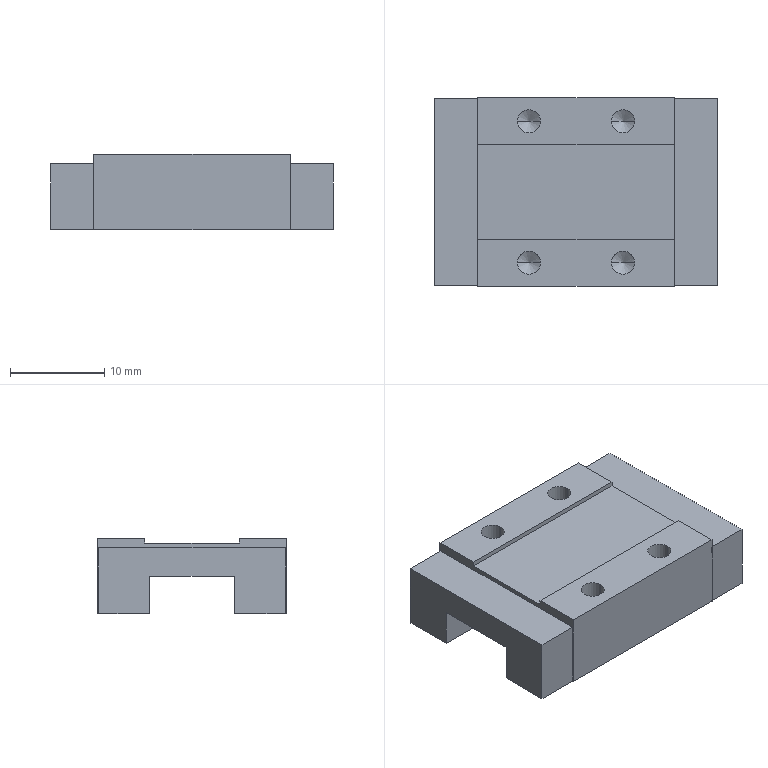Part | SolidWorks | features BaseBody 1 | 1 solid | 38 faces | box 30 x 20 x 8 mm | volume 3357 mm3 | plane 22 | cylinder 8 | cone 8 | commonest cylinder face diameters 2.459 x8
STEP:
#1=CARTESIAN_POINT('',(-38.836,-61.65,5.));
#2=VERTEX_POINT('',#1);
#3=CARTESIAN_POINT('',(-36.377,-61.65,5.));
#4=VERTEX_POINT('',#3);
#5=CARTESIAN_POINT('',(-37.606,-61.65,5.));
#6=DIRECTION('',(0.,0.,1.));
#7=DIRECTION('',(1.,0.,0.));
#8=AXIS2_PLACEMENT_3D('',#5,#6,#7);
#9=CIRCLE('',#8,1.23);
#10=EDGE_CURVE('',#2,#4,#9,.T.);
#11=ORIENTED_EDGE('',*,*,#10,.F.);
#12=CARTESIAN_POINT('',(-38.836,-61.65,8.));
#13=VERTEX_POINT('',#12);
#14=CARTESIAN_POINT('',(-38.836,-61.65,6.5));
#15=DIRECTION('',(0.,0.,1.));
#16=VECTOR('',#15,1000.);
#17=LINE('',#14,#16);
#18=EDGE_CURVE('',#2,#13,#17,.T.);
#19=ORIENTED_EDGE('',*,*,#18,.T.);
#20=CARTESIAN_POINT('',(-36.377,-61.65,8.));
#21=VERTEX_POINT('',#20);
#22=CARTESIAN_POINT('',(-37.606,-61.65,8.));
#23=DIRECTION('',(0.,0.,-1.));
#24=DIRECTION('',(1.,0.,0.));
#25=AXIS2_PLACEMENT_3D('',#22,#23,#24);
#26=CIRCLE('',#25,1.23);
#27=EDGE_CURVE('',#21,#13,#26,.T.);
#28=ORIENTED_EDGE('',*,*,#27,.F.);
#29=CARTESIAN_POINT('',(-36.377,-61.65,6.5));
#30=DIRECTION('',(0.,0.,1.));
#31=VECTOR('',#30,1000.);
#32=LINE('',#29,#31);
#33=EDGE_CURVE('',#4,#21,#32,.T.);
#34=ORIENTED_EDGE('',*,*,#33,.F.);
#35=EDGE_LOOP('',(#11,#19,#28,#34));
#36=FACE_OUTER_BOUND('',#35,.T.);
#37=CARTESIAN_POINT('',(-37.606,-61.65,6.5));
#38=DIRECTION('',(0.,0.,1.));
#39=DIRECTION('',(1.,0.,0.));
#40=AXIS2_PLACEMENT_3D('',#37,#38,#39);
#41=CYLINDRICAL_SURFACE('',#40,1.23);
#42=ADVANCED_FACE('',(#36),#41,.F.);
#43=CARTESIAN_POINT('',(-28.836,-61.65,5.));
#44=VERTEX_POINT('',#43);
#45=CARTESIAN_POINT('',(-26.377,-61.65,5.));
#46=VERTEX_POINT('',#45);
#47=CARTESIAN_POINT('',(-27.606,-61.65,5.));
#48=DIRECTION('',(0.,0.,1.));
#49=DIRECTION('',(1.,0.,0.));
#50=AXIS2_PLACEMENT_3D('',#47,#48,#49);
#51=CIRCLE('',#50,1.23);
#52=EDGE_CURVE('',#44,#46,#51,.T.);
#53=ORIENTED_EDGE('',*,*,#52,.F.);
#54=CARTESIAN_POINT('',(-28.836,-61.65,8.));
#55=VERTEX_POINT('',#54);
#56=CARTESIAN_POINT('',(-28.836,-61.65,6.5));
#57=DIRECTION('',(0.,0.,1.));
#58=VECTOR('',#57,1000.);
#59=LINE('',#56,#58);
#60=EDGE_CURVE('',#44,#55,#59,.T.);
#61=ORIENTED_EDGE('',*,*,#60,.T.);
#62=CARTESIAN_POINT('',(-26.377,-61.65,8.));
#63=VERTEX_POINT('',#62);
#64=CARTESIAN_POINT('',(-27.606,-61.65,8.));
#65=DIRECTION('',(0.,0.,-1.));
#66=DIRECTION('',(1.,0.,0.));
#67=AXIS2_PLACEMENT_3D('',#64,#65,#66);
#68=CIRCLE('',#67,1.23);
#69=EDGE_CURVE('',#63,#55,#68,.T.);
#70=ORIENTED_EDGE('',*,*,#69,.F.);
#71=CARTESIAN_POINT('',(-26.377,-61.65,6.5));
#72=DIRECTION('',(0.,0.,1.));
#73=VECTOR('',#72,1000.);
#74=LINE('',#71,#73);
#75=EDGE_CURVE('',#46,#63,#74,.T.);
#76=ORIENTED_EDGE('',*,*,#75,.F.);
#77=EDGE_LOOP('',(#53,#61,#70,#76));
#78=FACE_OUTER_BOUND('',#77,.T.);
#79=CARTESIAN_POINT('',(-27.606,-61.65,6.5));
#80=DIRECTION('',(0.,0.,1.));
#81=DIRECTION('',(1.,0.,0.));
#82=AXIS2_PLACEMENT_3D('',#79,#80,#81);
#83=CYLINDRICAL_SURFACE('',#82,1.23);
#84=ADVANCED_FACE('',(#78),#83,.F.);
#85=CARTESIAN_POINT('',(-38.836,-46.65,5.));
#86=VERTEX_POINT('',#85);
#87=CARTESIAN_POINT('',(-36.377,-46.65,5.));
#88=VERTEX_POINT('',#87);
#89=CARTESIAN_POINT('',(-37.606,-46.65,5.));
#90=DIRECTION('',(0.,0.,1.));
#91=DIRECTION('',(1.,0.,0.));
#92=AXIS2_PLACEMENT_3D('',#89,#90,#91);
#93=CIRCLE('',#92,1.23);
#94=EDGE_CURVE('',#86,#88,#93,.T.);
#95=ORIENTED_EDGE('',*,*,#94,.F.);
#96=CARTESIAN_POINT('',(-38.836,-46.65,8.));
#97=VERTEX_POINT('',#96);
#98=CARTESIAN_POINT('',(-38.836,-46.65,6.5));
#99=DIRECTION('',(0.,0.,1.));
#100=VECTOR('',#99,1000.);
#101=LINE('',#98,#100);
#102=EDGE_CURVE('',#86,#97,#101,.T.);
#103=ORIENTED_EDGE('',*,*,#102,.T.);
#104=CARTESIAN_POINT('',(-36.377,-46.65,8.));
#105=VERTEX_POINT('',#104);
#106=CARTESIAN_POINT('',(-37.606,-46.65,8.));
#107=DIRECTION('',(0.,0.,-1.));
#108=DIRECTION('',(1.,0.,0.));
#109=AXIS2_PLACEMENT_3D('',#106,#107,#108);
#110=CIRCLE('',#109,1.23);
#111=EDGE_CURVE('',#105,#97,#110,.T.);
#112=ORIENTED_EDGE('',*,*,#111,.F.);
#113=CARTESIAN_POINT('',(-36.377,-46.65,6.5));
#114=DIRECTION('',(0.,0.,1.));
#115=VECTOR('',#114,1000.);
#116=LINE('',#113,#115);
#117=EDGE_CURVE('',#88,#105,#116,.T.);
#118=ORIENTED_EDGE('',*,*,#117,.F.);
#119=EDGE_LOOP('',(#95,#103,#112,#118));
#120=FACE_OUTER_BOUND('',#119,.T.);
#121=CARTESIAN_POINT('',(-37.606,-46.65,6.5));
#122=DIRECTION('',(0.,0.,1.));
#123=DIRECTION('',(1.,0.,0.));
#124=AXIS2_PLACEMENT_3D('',#121,#122,#123);
#125=CYLINDRICAL_SURFACE('',#124,1.23);
#126=ADVANCED_FACE('',(#120),#125,.F.);
#127=CARTESIAN_POINT('',(-28.836,-46.65,5.));
#128=VERTEX_POINT('',#127);
#129=CARTESIAN_POINT('',(-26.377,-46.65,5.));
#130=VERTEX_POINT('',#129);
#131=CARTESIAN_POINT('',(-27.606,-46.65,5.));
#132=DIRECTION('',(0.,0.,1.));
#133=DIRECTION('',(1.,0.,0.));
#134=AXIS2_PLACEMENT_3D('',#131,#132,#133);
#135=CIRCLE('',#134,1.23);
#136=EDGE_CURVE('',#128,#130,#135,.T.);
#137=ORIENTED_EDGE('',*,*,#136,.F.);
#138=CARTESIAN_POINT('',(-28.836,-46.65,8.));
#139=VERTEX_POINT('',#138);
#140=CARTESIAN_POINT('',(-28.836,-46.65,6.5));
#141=DIRECTION('',(0.,0.,1.));
#142=VECTOR('',#141,1000.);
#143=LINE('',#140,#142);
#144=EDGE_CURVE('',#128,#139,#143,.T.);
#145=ORIENTED_EDGE('',*,*,#144,.T.);
#146=CARTESIAN_POINT('',(-26.377,-46.65,8.));
#147=VERTEX_POINT('',#146);
#148=CARTESIAN_POINT('',(-27.606,-46.65,8.));
#149=DIRECTION('',(0.,0.,-1.));
#150=DIRECTION('',(1.,0.,0.));
#151=AXIS2_PLACEMENT_3D('',#148,#149,#150);
#152=CIRCLE('',#151,1.23);
#153=EDGE_CURVE('',#147,#139,#152,.T.);
#154=ORIENTED_EDGE('',*,*,#153,.F.);
#155=CARTESIAN_POINT('',(-26.377,-46.65,6.5));
#156=DIRECTION('',(0.,0.,1.));
#157=VECTOR('',#156,1000.);
#158=LINE('',#155,#157);
#159=EDGE_CURVE('',#130,#147,#158,.T.);
#160=ORIENTED_EDGE('',*,*,#159,.F.);
#161=EDGE_LOOP('',(#137,#145,#154,#160));
#162=FACE_OUTER_BOUND('',#161,.T.);
#163=CARTESIAN_POINT('',(-27.606,-46.65,6.5));
#164=DIRECTION('',(0.,0.,1.));
#165=DIRECTION('',(1.,0.,0.));
#166=AXIS2_PLACEMENT_3D('',#163,#164,#165);
#167=CYLINDRICAL_SURFACE('',#166,1.23);
#168=ADVANCED_FACE('',(#162),#167,.F.);
#169=CARTESIAN_POINT('',(-37.606,-61.65,4.261));
#170=VERTEX_POINT('',#169);
#171=CARTESIAN_POINT('',(-36.377,-61.65,5.));
#172=DIRECTION('',(0.8572,0.,0.515));
#173=VECTOR('',#172,1000.);
#174=LINE('',#171,#173);
#175=EDGE_CURVE('',#170,#4,#174,.T.);
#176=ORIENTED_EDGE('',*,*,#175,.F.);
#177=CARTESIAN_POINT('',(-38.836,-61.65,5.));
#178=DIRECTION('',(-0.8572,0.,0.515));
#179=VECTOR('',#178,1000.);
#180=LINE('',#177,#179);
#181=EDGE_CURVE('',#170,#2,#180,.T.);
#182=ORIENTED_EDGE('',*,*,#181,.T.);
#183=ORIENTED_EDGE('',*,*,#10,.T.);
#184=EDGE_LOOP('',(#176,#182,#183));
#185=FACE_OUTER_BOUND('',#184,.T.);
#186=CARTESIAN_POINT('',(-37.606,-61.65,5.));
#187=DIRECTION('',(0.,0.,1.));
#188=DIRECTION('',(1.,0.,0.));
#189=AXIS2_PLACEMENT_3D('',#186,#187,#188);
#190=CONICAL_SURFACE('',#189,1.229,1.03);
#191=ADVANCED_FACE('',(#185),#190,.F.);
#192=CARTESIAN_POINT('',(-27.606,-61.65,4.261));
#193=VERTEX_POINT('',#192);
#194=CARTESIAN_POINT('',(-26.377,-61.65,5.));
#195=DIRECTION('',(0.8572,0.,0.515));
#196=VECTOR('',#195,1000.);
#197=LINE('',#194,#196);
#198=EDGE_CURVE('',#193,#46,#197,.T.);
#199=ORIENTED_EDGE('',*,*,#198,.F.);
#200=CARTESIAN_POINT('',(-28.836,-61.65,5.));
#201=DIRECTION('',(-0.8572,0.,0.515));
#202=VECTOR('',#201,1000.);
#203=LINE('',#200,#202);
#204=EDGE_CURVE('',#193,#44,#203,.T.);
#205=ORIENTED_EDGE('',*,*,#204,.T.);
#206=ORIENTED_EDGE('',*,*,#52,.T.);
#207=EDGE_LOOP('',(#199,#205,#206));
#208=FACE_OUTER_BOUND('',#207,.T.);
#209=CARTESIAN_POINT('',(-27.606,-61.65,5.));
#210=DIRECTION('',(0.,0.,1.));
#211=DIRECTION('',(1.,0.,0.));
#212=AXIS2_PLACEMENT_3D('',#209,#210,#211);
#213=CONICAL_SURFACE('',#212,1.229,1.03);
#214=ADVANCED_FACE('',(#208),#213,.F.);
#215=CARTESIAN_POINT('',(-37.606,-46.65,4.261));
#216=VERTEX_POINT('',#215);
#217=CARTESIAN_POINT('',(-36.377,-46.65,5.));
#218=DIRECTION('',(0.8572,0.,0.515));
#219=VECTOR('',#218,1000.);
#220=LINE('',#217,#219);
#221=EDGE_CURVE('',#216,#88,#220,.T.);
#222=ORIENTED_EDGE('',*,*,#221,.F.);
#223=CARTESIAN_POINT('',(-38.836,-46.65,5.));
#224=DIRECTION('',(-0.8572,0.,0.515));
#225=VECTOR('',#224,1000.);
#226=LINE('',#223,#225);
#227=EDGE_CURVE('',#216,#86,#226,.T.);
#228=ORIENTED_EDGE('',*,*,#227,.T.);
#229=ORIENTED_EDGE('',*,*,#94,.T.);
#230=EDGE_LOOP('',(#222,#228,#229));
#231=FACE_OUTER_BOUND('',#230,.T.);
#232=CARTESIAN_POINT('',(-37.606,-46.65,5.));
#233=DIRECTION('',(0.,0.,1.));
#234=DIRECTION('',(1.,0.,0.));
#235=AXIS2_PLACEMENT_3D('',#232,#233,#234);
#236=CONICAL_SURFACE('',#235,1.229,1.03);
#237=ADVANCED_FACE('',(#231),#236,.F.);
#238=CARTESIAN_POINT('',(-27.606,-46.65,4.261));
#239=VERTEX_POINT('',#238);
#240=CARTESIAN_POINT('',(-26.377,-46.65,5.));
#241=DIRECTION('',(0.8572,0.,0.515));
#242=VECTOR('',#241,1000.);
#243=LINE('',#240,#242);
#244=EDGE_CURVE('',#239,#130,#243,.T.);
#245=ORIENTED_EDGE('',*,*,#244,.F.);
#246=CARTESIAN_POINT('',(-28.836,-46.65,5.));
#247=DIRECTION('',(-0.8572,0.,0.515));
#248=VECTOR('',#247,1000.);
#249=LINE('',#246,#248);
#250=EDGE_CURVE('',#239,#128,#249,.T.);
#251=ORIENTED_EDGE('',*,*,#250,.T.);
#252=ORIENTED_EDGE('',*,*,#136,.T.);
#253=EDGE_LOOP('',(#245,#251,#252));
#254=FACE_OUTER_BOUND('',#253,.T.);
#255=CARTESIAN_POINT('',(-27.606,-46.65,5.));
#256=DIRECTION('',(0.,0.,1.));
#257=DIRECTION('',(1.,0.,0.));
#258=AXIS2_PLACEMENT_3D('',#255,#256,#257);
#259=CONICAL_SURFACE('',#258,1.229,1.03);
#260=ADVANCED_FACE('',(#254),#259,.F.);
#261=CARTESIAN_POINT('',(-47.606,-49.65,4.));
#262=VERTEX_POINT('',#261);
#263=CARTESIAN_POINT('',(-47.606,-58.65,4.));
#264=VERTEX_POINT('',#263);
#265=CARTESIAN_POINT('',(-47.606,-54.15,4.));
#266=DIRECTION('',(0.,-1.,0.));
#267=VECTOR('',#266,1000.);
#268=LINE('',#265,#267);
#269=EDGE_CURVE('',#262,#264,#268,.T.);
#270=ORIENTED_EDGE('',*,*,#269,.F.);
#271=CARTESIAN_POINT('',(-17.606,-49.65,4.));
#272=VERTEX_POINT('',#271);
#273=CARTESIAN_POINT('',(-32.606,-49.65,4.));
#274=DIRECTION('',(-1.,0.,0.));
#275=VECTOR('',#274,1000.);
#276=LINE('',#273,#275);
#277=EDGE_CURVE('',#272,#262,#276,.T.);
#278=ORIENTED_EDGE('',*,*,#277,.F.);
#279=CARTESIAN_POINT('',(-17.606,-58.65,4.));
#280=VERTEX_POINT('',#279);
#281=CARTESIAN_POINT('',(-17.606,-54.15,4.));
#282=DIRECTION('',(0.,1.,0.));
#283=VECTOR('',#282,1000.);
#284=LINE('',#281,#283);
#285=EDGE_CURVE('',#280,#272,#284,.T.);
#286=ORIENTED_EDGE('',*,*,#285,.F.);
#287=CARTESIAN_POINT('',(-32.606,-58.65,4.));
#288=DIRECTION('',(1.,0.,0.));
#289=VECTOR('',#288,1000.);
#290=LINE('',#287,#289);
#291=EDGE_CURVE('',#264,#280,#290,.T.);
#292=ORIENTED_EDGE('',*,*,#291,.F.);
#293=EDGE_LOOP('',(#270,#278,#286,#292));
#294=FACE_OUTER_BOUND('',#293,.T.);
#295=CARTESIAN_POINT('',(-32.606,-54.15,4.));
#296=DIRECTION('',(0.,0.,1.));
#297=DIRECTION('',(1.,0.,0.));
#298=AXIS2_PLACEMENT_3D('',#295,#296,#297);
#299=PLANE('',#298);
#300=ADVANCED_FACE('',(#294),#299,.F.);
#301=CARTESIAN_POINT('',(-17.606,-58.65,0.));
#302=VERTEX_POINT('',#301);
#303=CARTESIAN_POINT('',(-17.606,-58.65,0.));
#304=DIRECTION('',(0.,0.,1.));
#305=VECTOR('',#304,1000.);
#306=LINE('',#303,#305);
#307=EDGE_CURVE('',#302,#280,#306,.T.);
#308=ORIENTED_EDGE('',*,*,#307,.F.);
#309=CARTESIAN_POINT('',(-47.606,-58.65,0.));
#310=VERTEX_POINT('',#309);
#311=CARTESIAN_POINT('',(-17.606,-58.65,0.));
#312=DIRECTION('',(1.,0.,0.));
#313=VECTOR('',#312,1000.);
#314=LINE('',#311,#313);
#315=EDGE_CURVE('',#310,#302,#314,.T.);
#316=ORIENTED_EDGE('',*,*,#315,.F.);
#317=CARTESIAN_POINT('',(-47.606,-58.65,0.));
#318=DIRECTION('',(0.,0.,-1.));
#319=VECTOR('',#318,1000.);
#320=LINE('',#317,#319);
#321=EDGE_CURVE('',#264,#310,#320,.T.);
#322=ORIENTED_EDGE('',*,*,#321,.F.);
#323=ORIENTED_EDGE('',*,*,#291,.T.);
#324=EDGE_LOOP('',(#308,#316,#322,#323));
#325=FACE_OUTER_BOUND('',#324,.T.);
#326=CARTESIAN_POINT('',(-17.606,-58.65,0.));
#327=DIRECTION('',(0.,-1.,0.));
#328=DIRECTION('',(0.,0.,-1.));
#329=AXIS2_PLACEMENT_3D('',#326,#327,#328);
#330=PLANE('',#329);
#331=ADVANCED_FACE('',(#325),#330,.F.);
#332=CARTESIAN_POINT('',(-47.606,-64.05,0.));
#333=VERTEX_POINT('',#332);
#334=CARTESIAN_POINT('',(-47.606,-64.05,7.));
#335=VERTEX_POINT('',#334);
#336=CARTESIAN_POINT('',(-47.606,-64.05,0.));
#337=DIRECTION('',(0.,0.,1.));
#338=VECTOR('',#337,1000.);
#339=LINE('',#336,#338);
#340=EDGE_CURVE('',#333,#335,#339,.T.);
#341=ORIENTED_EDGE('',*,*,#340,.T.);
#342=CARTESIAN_POINT('',(-47.606,-44.25,7.));
#343=VERTEX_POINT('',#342);
#344=CARTESIAN_POINT('',(-47.606,-64.15,7.));
#345=DIRECTION('',(0.,1.,0.));
#346=VECTOR('',#345,1000.);
#347=LINE('',#344,#346);
#348=EDGE_CURVE('',#335,#343,#347,.T.);
#349=ORIENTED_EDGE('',*,*,#348,.T.);
#350=CARTESIAN_POINT('',(-47.606,-44.25,0.));
#351=VERTEX_POINT('',#350);
#352=CARTESIAN_POINT('',(-47.606,-44.25,0.));
#353=DIRECTION('',(0.,0.,-1.));
#354=VECTOR('',#353,1000.);
#355=LINE('',#352,#354);
#356=EDGE_CURVE('',#343,#351,#355,.T.);
#357=ORIENTED_EDGE('',*,*,#356,.T.);
#358=CARTESIAN_POINT('',(-47.606,-49.65,0.));
#359=VERTEX_POINT('',#358);
#360=CARTESIAN_POINT('',(-47.606,-64.15,0.));
#361=DIRECTION('',(0.,-1.,0.));
#362=VECTOR('',#361,1000.);
#363=LINE('',#360,#362);
#364=EDGE_CURVE('',#351,#359,#363,.T.);
#365=ORIENTED_EDGE('',*,*,#364,.T.);
#366=CARTESIAN_POINT('',(-47.606,-49.65,0.));
#367=DIRECTION('',(0.,0.,1.));
#368=VECTOR('',#367,1000.);
#369=LINE('',#366,#368);
#370=EDGE_CURVE('',#359,#262,#369,.T.);
#371=ORIENTED_EDGE('',*,*,#370,.T.);
#372=ORIENTED_EDGE('',*,*,#269,.T.);
#373=ORIENTED_EDGE('',*,*,#321,.T.);
#374=CARTESIAN_POINT('',(-47.606,-64.15,0.));
#375=DIRECTION('',(0.,-1.,0.));
#376=VECTOR('',#375,1000.);
#377=LINE('',#374,#376);
#378=EDGE_CURVE('',#310,#333,#377,.T.);
#379=ORIENTED_EDGE('',*,*,#378,.T.);
#380=EDGE_LOOP('',(#341,#349,#357,#365,#371,#372,#373,#379));
#381=FACE_OUTER_BOUND('',#380,.T.);
#382=CARTESIAN_POINT('',(-47.606,-64.15,0.));
#383=DIRECTION('',(-1.,0.,0.));
#384=DIRECTION('',(0.,0.,1.));
#385=AXIS2_PLACEMENT_3D('',#382,#383,#384);
#386=PLANE('',#385);
#387=ADVANCED_FACE('',(#381),#386,.T.);
#388=ORIENTED_EDGE('',*,*,#370,.F.);
#389=CARTESIAN_POINT('',(-17.606,-49.65,0.));
#390=VERTEX_POINT('',#389);
#391=CARTESIAN_POINT('',(-47.606,-49.65,0.));
#392=DIRECTION('',(-1.,0.,0.));
#393=VECTOR('',#392,1000.);
#394=LINE('',#391,#393);
#395=EDGE_CURVE('',#390,#359,#394,.T.);
#396=ORIENTED_EDGE('',*,*,#395,.F.);
#397=CARTESIAN_POINT('',(-17.606,-49.65,0.));
#398=DIRECTION('',(0.,0.,-1.));
#399=VECTOR('',#398,1000.);
#400=LINE('',#397,#399);
#401=EDGE_CURVE('',#272,#390,#400,.T.);
#402=ORIENTED_EDGE('',*,*,#401,.F.);
#403=ORIENTED_EDGE('',*,*,#277,.T.);
#404=EDGE_LOOP('',(#388,#396,#402,#403));
#405=FACE_OUTER_BOUND('',#404,.T.);
#406=CARTESIAN_POINT('',(-47.606,-49.65,0.));
#407=DIRECTION('',(0.,1.,0.));
#408=DIRECTION('',(0.,0.,1.));
#409=AXIS2_PLACEMENT_3D('',#406,#407,#408);
#410=PLANE('',#409);
#411=ADVANCED_FACE('',(#405),#410,.F.);
#412=ORIENTED_EDGE('',*,*,#401,.T.);
#413=CARTESIAN_POINT('',(-17.606,-44.25,0.));
#414=VERTEX_POINT('',#413);
#415=CARTESIAN_POINT('',(-17.606,-44.15,0.));
#416=DIRECTION('',(0.,1.,0.));
#417=VECTOR('',#416,1000.);
#418=LINE('',#415,#417);
#419=EDGE_CURVE('',#390,#414,#418,.T.);
#420=ORIENTED_EDGE('',*,*,#419,.T.);
#421=CARTESIAN_POINT('',(-17.606,-44.25,7.));
#422=VERTEX_POINT('',#421);
#423=CARTESIAN_POINT('',(-17.606,-44.25,0.));
#424=DIRECTION('',(0.,0.,1.));
#425=VECTOR('',#424,1000.);
#426=LINE('',#423,#425);
#427=EDGE_CURVE('',#414,#422,#426,.T.);
#428=ORIENTED_EDGE('',*,*,#427,.T.);
#429=CARTESIAN_POINT('',(-17.606,-64.05,7.));
#430=VERTEX_POINT('',#429);
#431=CARTESIAN_POINT('',(-17.606,-44.15,7.));
#432=DIRECTION('',(0.,-1.,0.));
#433=VECTOR('',#432,1000.);
#434=LINE('',#431,#433);
#435=EDGE_CURVE('',#422,#430,#434,.T.);
#436=ORIENTED_EDGE('',*,*,#435,.T.);
#437=CARTESIAN_POINT('',(-17.606,-64.05,0.));
#438=VERTEX_POINT('',#437);
#439=CARTESIAN_POINT('',(-17.606,-64.05,0.));
#440=DIRECTION('',(0.,0.,-1.));
#441=VECTOR('',#440,1000.);
#442=LINE('',#439,#441);
#443=EDGE_CURVE('',#430,#438,#442,.T.);
#444=ORIENTED_EDGE('',*,*,#443,.T.);
#445=CARTESIAN_POINT('',(-17.606,-44.15,0.));
#446=DIRECTION('',(0.,1.,0.));
#447=VECTOR('',#446,1000.);
#448=LINE('',#445,#447);
#449=EDGE_CURVE('',#438,#302,#448,.T.);
#450=ORIENTED_EDGE('',*,*,#449,.T.);
#451=ORIENTED_EDGE('',*,*,#307,.T.);
#452=ORIENTED_EDGE('',*,*,#285,.T.);
#453=EDGE_LOOP('',(#412,#420,#428,#436,#444,#450,#451,#452));
#454=FACE_OUTER_BOUND('',#453,.T.);
#455=CARTESIAN_POINT('',(-17.606,-44.15,0.));
#456=DIRECTION('',(1.,0.,0.));
#457=DIRECTION('',(0.,0.,-1.));
#458=AXIS2_PLACEMENT_3D('',#455,#456,#457);
#459=PLANE('',#458);
#460=ADVANCED_FACE('',(#454),#459,.T.);
#461=ORIENTED_EDGE('',*,*,#378,.F.);
#462=ORIENTED_EDGE('',*,*,#315,.T.);
#463=ORIENTED_EDGE('',*,*,#449,.F.);
#464=CARTESIAN_POINT('',(-22.206,-64.05,0.));
#465=VERTEX_POINT('',#464);
#466=CARTESIAN_POINT('',(-32.606,-64.05,0.));
#467=DIRECTION('',(1.,0.,0.));
#468=VECTOR('',#467,1000.);
#469=LINE('',#466,#468);
#470=EDGE_CURVE('',#465,#438,#469,.T.);
#471=ORIENTED_EDGE('',*,*,#470,.F.);
#472=CARTESIAN_POINT('',(-22.206,-64.15,0.));
#473=VERTEX_POINT('',#472);
#474=CARTESIAN_POINT('',(-22.206,-44.15,0.));
#475=DIRECTION('',(0.,-1.,0.));
#476=VECTOR('',#475,1000.);
#477=LINE('',#474,#476);
#478=EDGE_CURVE('',#465,#473,#477,.T.);
#479=ORIENTED_EDGE('',*,*,#478,.T.);
#480=CARTESIAN_POINT('',(-43.006,-64.15,0.));
#481=VERTEX_POINT('',#480);
#482=CARTESIAN_POINT('',(-32.606,-64.15,0.));
#483=DIRECTION('',(1.,0.,0.));
#484=VECTOR('',#483,1000.);
#485=LINE('',#482,#484);
#486=EDGE_CURVE('',#481,#473,#485,.T.);
#487=ORIENTED_EDGE('',*,*,#486,.F.);
#488=CARTESIAN_POINT('',(-43.006,-64.05,0.));
#489=VERTEX_POINT('',#488);
#490=CARTESIAN_POINT('',(-43.006,-64.15,0.));
#491=DIRECTION('',(0.,1.,0.));
#492=VECTOR('',#491,1000.);
#493=LINE('',#490,#492);
#494=EDGE_CURVE('',#481,#489,#493,.T.);
#495=ORIENTED_EDGE('',*,*,#494,.T.);
#496=CARTESIAN_POINT('',(-32.606,-64.05,0.));
#497=DIRECTION('',(1.,0.,0.));
#498=VECTOR('',#497,1000.);
#499=LINE('',#496,#498);
#500=EDGE_CURVE('',#333,#489,#499,.T.);
#501=ORIENTED_EDGE('',*,*,#500,.F.);
#502=EDGE_LOOP('',(#461,#462,#463,#471,#479,#487,#495,#501));
#503=FACE_OUTER_BOUND('',#502,.T.);
#504=CARTESIAN_POINT('',(-32.606,-54.15,0.));
#505=DIRECTION('',(0.,0.,1.));
#506=DIRECTION('',(1.,0.,0.));
#507=AXIS2_PLACEMENT_3D('',#504,#505,#506);
#508=PLANE('',#507);
#509=ADVANCED_FACE('',(#503),#508,.F.);
#510=CARTESIAN_POINT('',(-43.006,-64.05,7.));
#511=VERTEX_POINT('',#510);
#512=CARTESIAN_POINT('',(-45.306,-64.05,7.));
#513=DIRECTION('',(1.,0.,0.));
#514=VECTOR('',#513,1000.);
#515=LINE('',#512,#514);
#516=EDGE_CURVE('',#335,#511,#515,.T.);
#517=ORIENTED_EDGE('',*,*,#516,.T.);
#518=CARTESIAN_POINT('',(-43.006,-44.25,7.));
#519=VERTEX_POINT('',#518);
#520=CARTESIAN_POINT('',(-43.006,-54.15,7.));
#521=DIRECTION('',(0.,1.,0.));
#522=VECTOR('',#521,1000.);
#523=LINE('',#520,#522);
#524=EDGE_CURVE('',#511,#519,#523,.T.);
#525=ORIENTED_EDGE('',*,*,#524,.T.);
#526=CARTESIAN_POINT('',(-45.306,-44.25,7.));
#527=DIRECTION('',(-1.,0.,0.));
#528=VECTOR('',#527,1000.);
#529=LINE('',#526,#528);
#530=EDGE_CURVE('',#519,#343,#529,.T.);
#531=ORIENTED_EDGE('',*,*,#530,.T.);
#532=ORIENTED_EDGE('',*,*,#348,.F.);
#533=EDGE_LOOP('',(#517,#525,#531,#532));
#534=FACE_OUTER_BOUND('',#533,.T.);
#535=CARTESIAN_POINT('',(-45.306,-54.15,7.));
#536=DIRECTION('',(0.,0.,1.));
#537=DIRECTION('',(1.,0.,0.));
#538=AXIS2_PLACEMENT_3D('',#535,#536,#537);
#539=PLANE('',#538);
#540=ADVANCED_FACE('',(#534),#539,.T.);
#541=ORIENTED_EDGE('',*,*,#500,.T.);
#542=CARTESIAN_POINT('',(-43.006,-64.05,3.5));
#543=DIRECTION('',(0.,0.,-1.));
#544=VECTOR('',#543,1000.);
#545=LINE('',#542,#544);
#546=EDGE_CURVE('',#511,#489,#545,.T.);
#547=ORIENTED_EDGE('',*,*,#546,.F.);
#548=ORIENTED_EDGE('',*,*,#516,.F.);
#549=ORIENTED_EDGE('',*,*,#340,.F.);
#550=EDGE_LOOP('',(#541,#547,#548,#549));
#551=FACE_OUTER_BOUND('',#550,.T.);
#552=CARTESIAN_POINT('',(-45.306,-64.05,3.5));
#553=DIRECTION('',(0.,1.,0.));
#554=DIRECTION('',(0.,0.,1.));
#555=AXIS2_PLACEMENT_3D('',#552,#553,#554);
#556=PLANE('',#555);
#557=ADVANCED_FACE('',(#551),#556,.F.);
#558=CARTESIAN_POINT('',(-43.006,-44.15,0.));
#559=VERTEX_POINT('',#558);
#560=CARTESIAN_POINT('',(-43.006,-44.25,0.));
#561=VERTEX_POINT('',#560);
#562=CARTESIAN_POINT('',(-43.006,-54.15,0.));
#563=DIRECTION('',(0.,-1.,0.));
#564=VECTOR('',#563,1000.);
#565=LINE('',#562,#564);
#566=EDGE_CURVE('',#559,#561,#565,.T.);
#567=ORIENTED_EDGE('',*,*,#566,.F.);
#568=CARTESIAN_POINT('',(-22.206,-44.15,0.));
#569=VERTEX_POINT('',#568);
#570=CARTESIAN_POINT('',(-32.606,-44.15,0.));
#571=DIRECTION('',(-1.,0.,0.));
#572=VECTOR('',#571,1000.);
#573=LINE('',#570,#572);
#574=EDGE_CURVE('',#569,#559,#573,.T.);
#575=ORIENTED_EDGE('',*,*,#574,.F.);
#576=CARTESIAN_POINT('',(-22.206,-44.25,0.));
#577=VERTEX_POINT('',#576);
#578=CARTESIAN_POINT('',(-22.206,-44.15,0.));
#579=DIRECTION('',(0.,-1.,0.));
#580=VECTOR('',#579,1000.);
#581=LINE('',#578,#580);
#582=EDGE_CURVE('',#569,#577,#581,.T.);
#583=ORIENTED_EDGE('',*,*,#582,.T.);
#584=CARTESIAN_POINT('',(-32.606,-44.25,0.));
#585=DIRECTION('',(-1.,0.,0.));
#586=VECTOR('',#585,1000.);
#587=LINE('',#584,#586);
#588=EDGE_CURVE('',#414,#577,#587,.T.);
#589=ORIENTED_EDGE('',*,*,#588,.F.);
#590=ORIENTED_EDGE('',*,*,#419,.F.);
#591=ORIENTED_EDGE('',*,*,#395,.T.);
#592=ORIENTED_EDGE('',*,*,#364,.F.);
#593=CARTESIAN_POINT('',(-32.606,-44.25,0.));
#594=DIRECTION('',(-1.,0.,0.));
#595=VECTOR('',#594,1000.);
#596=LINE('',#593,#595);
#597=EDGE_CURVE('',#561,#351,#596,.T.);
#598=ORIENTED_EDGE('',*,*,#597,.F.);
#599=EDGE_LOOP('',(#567,#575,#583,#589,#590,#591,#592,#598));
#600=FACE_OUTER_BOUND('',#599,.T.);
#601=CARTESIAN_POINT('',(-32.606,-54.15,0.));
#602=DIRECTION('',(0.,0.,1.));
#603=DIRECTION('',(1.,0.,0.));
#604=AXIS2_PLACEMENT_3D('',#601,#602,#603);
#605=PLANE('',#604);
#606=ADVANCED_FACE('',(#600),#605,.F.);
#607=ORIENTED_EDGE('',*,*,#530,.F.);
#608=CARTESIAN_POINT('',(-43.006,-44.25,3.5));
#609=DIRECTION('',(0.,0.,-1.));
#610=VECTOR('',#609,1000.);
#611=LINE('',#608,#610);
#612=EDGE_CURVE('',#519,#561,#611,.T.);
#613=ORIENTED_EDGE('',*,*,#612,.T.);
#614=ORIENTED_EDGE('',*,*,#597,.T.);
#615=ORIENTED_EDGE('',*,*,#356,.F.);
#616=EDGE_LOOP('',(#607,#613,#614,#615));
#617=FACE_OUTER_BOUND('',#616,.T.);
#618=CARTESIAN_POINT('',(-45.306,-44.25,3.5));
#619=DIRECTION('',(0.,1.,0.));
#620=DIRECTION('',(0.,0.,1.));
#621=AXIS2_PLACEMENT_3D('',#618,#619,#620);
#622=PLANE('',#621);
#623=ADVANCED_FACE('',(#617),#622,.T.);
#624=CARTESIAN_POINT('',(-22.206,-64.05,7.));
#625=VERTEX_POINT('',#624);
#626=CARTESIAN_POINT('',(-22.206,-64.05,3.5));
#627=DIRECTION('',(0.,0.,1.));
#628=VECTOR('',#627,1000.);
#629=LINE('',#626,#628);
#630=EDGE_CURVE('',#465,#625,#629,.T.);
#631=ORIENTED_EDGE('',*,*,#630,.F.);
#632=ORIENTED_EDGE('',*,*,#470,.T.);
#633=ORIENTED_EDGE('',*,*,#443,.F.);
#634=CARTESIAN_POINT('',(-19.906,-64.05,7.));
#635=DIRECTION('',(1.,0.,0.));
#636=VECTOR('',#635,1000.);
#637=LINE('',#634,#636);
#638=EDGE_CURVE('',#625,#430,#637,.T.);
#639=ORIENTED_EDGE('',*,*,#638,.F.);
#640=EDGE_LOOP('',(#631,#632,#633,#639));
#641=FACE_OUTER_BOUND('',#640,.T.);
#642=CARTESIAN_POINT('',(-19.906,-64.05,3.5));
#643=DIRECTION('',(0.,1.,0.));
#644=DIRECTION('',(0.,0.,1.));
#645=AXIS2_PLACEMENT_3D('',#642,#643,#644);
#646=PLANE('',#645);
#647=ADVANCED_FACE('',(#641),#646,.F.);
#648=ORIENTED_EDGE('',*,*,#638,.T.);
#649=ORIENTED_EDGE('',*,*,#435,.F.);
#650=CARTESIAN_POINT('',(-22.206,-44.25,7.));
#651=VERTEX_POINT('',#650);
#652=CARTESIAN_POINT('',(-19.906,-44.25,7.));
#653=DIRECTION('',(-1.,0.,0.));
#654=VECTOR('',#653,1000.);
#655=LINE('',#652,#654);
#656=EDGE_CURVE('',#422,#651,#655,.T.);
#657=ORIENTED_EDGE('',*,*,#656,.T.);
#658=CARTESIAN_POINT('',(-22.206,-54.15,7.));
#659=DIRECTION('',(0.,-1.,0.));
#660=VECTOR('',#659,1000.);
#661=LINE('',#658,#660);
#662=EDGE_CURVE('',#651,#625,#661,.T.);
#663=ORIENTED_EDGE('',*,*,#662,.T.);
#664=EDGE_LOOP('',(#648,#649,#657,#663));
#665=FACE_OUTER_BOUND('',#664,.T.);
#666=CARTESIAN_POINT('',(-19.906,-54.15,7.));
#667=DIRECTION('',(0.,0.,1.));
#668=DIRECTION('',(1.,0.,0.));
#669=AXIS2_PLACEMENT_3D('',#666,#667,#668);
#670=PLANE('',#669);
#671=ADVANCED_FACE('',(#665),#670,.T.);
#672=CARTESIAN_POINT('',(-22.206,-44.25,3.5));
#673=DIRECTION('',(0.,0.,1.));
#674=VECTOR('',#673,1000.);
#675=LINE('',#672,#674);
#676=EDGE_CURVE('',#577,#651,#675,.T.);
#677=ORIENTED_EDGE('',*,*,#676,.T.);
#678=ORIENTED_EDGE('',*,*,#656,.F.);
#679=ORIENTED_EDGE('',*,*,#427,.F.);
#680=ORIENTED_EDGE('',*,*,#588,.T.);
#681=EDGE_LOOP('',(#677,#678,#679,#680));
#682=FACE_OUTER_BOUND('',#681,.T.);
#683=CARTESIAN_POINT('',(-19.906,-44.25,3.5));
#684=DIRECTION('',(0.,1.,0.));
#685=DIRECTION('',(0.,0.,1.));
#686=AXIS2_PLACEMENT_3D('',#683,#684,#685);
#687=PLANE('',#686);
#688=ADVANCED_FACE('',(#682),#687,.T.);
#689=CARTESIAN_POINT('',(-22.206,-64.15,8.));
#690=VERTEX_POINT('',#689);
#691=CARTESIAN_POINT('',(-22.206,-64.15,0.));
#692=DIRECTION('',(0.,0.,1.));
#693=VECTOR('',#692,1000.);
#694=LINE('',#691,#693);
#695=EDGE_CURVE('',#473,#690,#694,.T.);
#696=ORIENTED_EDGE('',*,*,#695,.T.);
#697=CARTESIAN_POINT('',(-43.006,-64.15,8.));
#698=VERTEX_POINT('',#697);
#699=CARTESIAN_POINT('',(-17.606,-64.15,8.));
#700=DIRECTION('',(-1.,0.,0.));
#701=VECTOR('',#700,1000.);
#702=LINE('',#699,#701);
#703=EDGE_CURVE('',#690,#698,#702,.T.);
#704=ORIENTED_EDGE('',*,*,#703,.T.);
#705=CARTESIAN_POINT('',(-43.006,-64.15,0.));
#706=DIRECTION('',(0.,0.,-1.));
#707=VECTOR('',#706,1000.);
#708=LINE('',#705,#707);
#709=EDGE_CURVE('',#698,#481,#708,.T.);
#710=ORIENTED_EDGE('',*,*,#709,.T.);
#711=ORIENTED_EDGE('',*,*,#486,.T.);
#712=EDGE_LOOP('',(#696,#704,#710,#711));
#713=FACE_OUTER_BOUND('',#712,.T.);
#714=CARTESIAN_POINT('',(-17.606,-64.15,0.));
#715=DIRECTION('',(0.,-1.,0.));
#716=DIRECTION('',(0.,0.,-1.));
#717=AXIS2_PLACEMENT_3D('',#714,#715,#716);
#718=PLANE('',#717);
#719=ADVANCED_FACE('',(#713),#718,.T.);
#720=CARTESIAN_POINT('',(-43.006,-49.15,7.5));
#721=VERTEX_POINT('',#720);
#722=CARTESIAN_POINT('',(-43.006,-59.15,7.5));
#723=VERTEX_POINT('',#722);
#724=CARTESIAN_POINT('',(-43.006,-64.15,7.5));
#725=DIRECTION('',(0.,-1.,0.));
#726=VECTOR('',#725,1000.);
#727=LINE('',#724,#726);
#728=EDGE_CURVE('',#721,#723,#727,.T.);
#729=ORIENTED_EDGE('',*,*,#728,.F.);
#730=CARTESIAN_POINT('',(-43.006,-49.15,8.));
#731=VERTEX_POINT('',#730);
#732=CARTESIAN_POINT('',(-43.006,-49.15,8.));
#733=DIRECTION('',(0.,0.,1.));
#734=VECTOR('',#733,1000.);
#735=LINE('',#732,#734);
#736=EDGE_CURVE('',#721,#731,#735,.T.);
#737=ORIENTED_EDGE('',*,*,#736,.T.);
#738=CARTESIAN_POINT('',(-43.006,-44.15,8.));
#739=VERTEX_POINT('',#738);
#740=CARTESIAN_POINT('',(-43.006,-64.15,8.));
#741=DIRECTION('',(0.,-1.,0.));
#742=VECTOR('',#741,1000.);
#743=LINE('',#740,#742);
#744=EDGE_CURVE('',#739,#731,#743,.T.);
#745=ORIENTED_EDGE('',*,*,#744,.F.);
#746=CARTESIAN_POINT('',(-43.006,-44.15,8.));
#747=DIRECTION('',(0.,0.,1.));
#748=VECTOR('',#747,1000.);
#749=LINE('',#746,#748);
#750=EDGE_CURVE('',#559,#739,#749,.T.);
#751=ORIENTED_EDGE('',*,*,#750,.F.);
#752=ORIENTED_EDGE('',*,*,#566,.T.);
#753=ORIENTED_EDGE('',*,*,#612,.F.);
#754=ORIENTED_EDGE('',*,*,#524,.F.);
#755=ORIENTED_EDGE('',*,*,#546,.T.);
#756=ORIENTED_EDGE('',*,*,#494,.F.);
#757=ORIENTED_EDGE('',*,*,#709,.F.);
#758=CARTESIAN_POINT('',(-43.006,-59.15,8.));
#759=VERTEX_POINT('',#758);
#760=CARTESIAN_POINT('',(-43.006,-64.15,8.));
#761=DIRECTION('',(0.,-1.,0.));
#762=VECTOR('',#761,1000.);
#763=LINE('',#760,#762);
#764=EDGE_CURVE('',#759,#698,#763,.T.);
#765=ORIENTED_EDGE('',*,*,#764,.F.);
#766=CARTESIAN_POINT('',(-43.006,-59.15,8.));
#767=DIRECTION('',(0.,0.,-1.));
#768=VECTOR('',#767,1000.);
#769=LINE('',#766,#768);
#770=EDGE_CURVE('',#759,#723,#769,.T.);
#771=ORIENTED_EDGE('',*,*,#770,.T.);
#772=EDGE_LOOP('',(#729,#737,#745,#751,#752,#753,#754,#755,#756,#757,#765,#771));
#773=FACE_OUTER_BOUND('',#772,.T.);
#774=CARTESIAN_POINT('',(-43.006,-64.15,8.));
#775=DIRECTION('',(1.,0.,0.));
#776=DIRECTION('',(0.,0.,-1.));
#777=AXIS2_PLACEMENT_3D('',#774,#775,#776);
#778=PLANE('',#777);
#779=ADVANCED_FACE('',(#773),#778,.F.);
#780=CARTESIAN_POINT('',(-22.206,-44.15,8.));
#781=VERTEX_POINT('',#780);
#782=CARTESIAN_POINT('',(-22.206,-44.15,0.));
#783=DIRECTION('',(0.,0.,-1.));
#784=VECTOR('',#783,1000.);
#785=LINE('',#782,#784);
#786=EDGE_CURVE('',#781,#569,#785,.T.);
#787=ORIENTED_EDGE('',*,*,#786,.T.);
#788=ORIENTED_EDGE('',*,*,#574,.T.);
#789=ORIENTED_EDGE('',*,*,#750,.T.);
#790=CARTESIAN_POINT('',(-47.606,-44.15,8.));
#791=DIRECTION('',(1.,0.,0.));
#792=VECTOR('',#791,1000.);
#793=LINE('',#790,#792);
#794=EDGE_CURVE('',#739,#781,#793,.T.);
#795=ORIENTED_EDGE('',*,*,#794,.T.);
#796=EDGE_LOOP('',(#787,#788,#789,#795));
#797=FACE_OUTER_BOUND('',#796,.T.);
#798=CARTESIAN_POINT('',(-47.606,-44.15,0.));
#799=DIRECTION('',(0.,1.,0.));
#800=DIRECTION('',(0.,0.,1.));
#801=AXIS2_PLACEMENT_3D('',#798,#799,#800);
#802=PLANE('',#801);
#803=ADVANCED_FACE('',(#797),#802,.T.);
#804=CARTESIAN_POINT('',(-22.206,-59.15,8.));
#805=VERTEX_POINT('',#804);
#806=CARTESIAN_POINT('',(-22.206,-44.15,8.));
#807=DIRECTION('',(0.,1.,0.));
#808=VECTOR('',#807,1000.);
#809=LINE('',#806,#808);
#810=EDGE_CURVE('',#690,#805,#809,.T.);
#811=ORIENTED_EDGE('',*,*,#810,.F.);
#812=ORIENTED_EDGE('',*,*,#695,.F.);
#813=ORIENTED_EDGE('',*,*,#478,.F.);
#814=ORIENTED_EDGE('',*,*,#630,.T.);
#815=ORIENTED_EDGE('',*,*,#662,.F.);
#816=ORIENTED_EDGE('',*,*,#676,.F.);
#817=ORIENTED_EDGE('',*,*,#582,.F.);
#818=ORIENTED_EDGE('',*,*,#786,.F.);
#819=CARTESIAN_POINT('',(-22.206,-49.15,8.));
#820=VERTEX_POINT('',#819);
#821=CARTESIAN_POINT('',(-22.206,-44.15,8.));
#822=DIRECTION('',(0.,1.,0.));
#823=VECTOR('',#822,1000.);
#824=LINE('',#821,#823);
#825=EDGE_CURVE('',#820,#781,#824,.T.);
#826=ORIENTED_EDGE('',*,*,#825,.F.);
#827=CARTESIAN_POINT('',(-22.206,-49.15,7.5));
#828=VERTEX_POINT('',#827);
#829=CARTESIAN_POINT('',(-22.206,-49.15,8.));
#830=DIRECTION('',(0.,0.,-1.));
#831=VECTOR('',#830,1000.);
#832=LINE('',#829,#831);
#833=EDGE_CURVE('',#820,#828,#832,.T.);
#834=ORIENTED_EDGE('',*,*,#833,.T.);
#835=CARTESIAN_POINT('',(-22.206,-59.15,7.5));
#836=VERTEX_POINT('',#835);
#837=CARTESIAN_POINT('',(-22.206,-44.15,7.5));
#838=DIRECTION('',(0.,1.,0.));
#839=VECTOR('',#838,1000.);
#840=LINE('',#837,#839);
#841=EDGE_CURVE('',#836,#828,#840,.T.);
#842=ORIENTED_EDGE('',*,*,#841,.F.);
#843=CARTESIAN_POINT('',(-22.206,-59.15,8.));
#844=DIRECTION('',(0.,0.,1.));
#845=VECTOR('',#844,1000.);
#846=LINE('',#843,#845);
#847=EDGE_CURVE('',#836,#805,#846,.T.);
#848=ORIENTED_EDGE('',*,*,#847,.T.);
#849=EDGE_LOOP('',(#811,#812,#813,#814,#815,#816,#817,#818,#826,#834,#842,#848));
#850=FACE_OUTER_BOUND('',#849,.T.);
#851=CARTESIAN_POINT('',(-22.206,-44.15,8.));
#852=DIRECTION('',(-1.,0.,0.));
#853=DIRECTION('',(0.,0.,1.));
#854=AXIS2_PLACEMENT_3D('',#851,#852,#853);
#855=PLANE('',#854);
#856=ADVANCED_FACE('',(#850),#855,.F.);
#857=ORIENTED_EDGE('',*,*,#27,.T.);
#858=CARTESIAN_POINT('',(-37.606,-61.65,8.));
#859=DIRECTION('',(0.,0.,-1.));
#860=DIRECTION('',(1.,0.,0.));
#861=AXIS2_PLACEMENT_3D('',#858,#859,#860);
#862=CIRCLE('',#861,1.23);
#863=EDGE_CURVE('',#13,#21,#862,.T.);
#864=ORIENTED_EDGE('',*,*,#863,.T.);
#865=EDGE_LOOP('',(#857,#864));
#866=FACE_BOUND('',#865,.T.);
#867=ORIENTED_EDGE('',*,*,#69,.T.);
#868=CARTESIAN_POINT('',(-27.606,-61.65,8.));
#869=DIRECTION('',(0.,0.,-1.));
#870=DIRECTION('',(1.,0.,0.));
#871=AXIS2_PLACEMENT_3D('',#868,#869,#870);
#872=CIRCLE('',#871,1.23);
#873=EDGE_CURVE('',#55,#63,#872,.T.);
#874=ORIENTED_EDGE('',*,*,#873,.T.);
#875=EDGE_LOOP('',(#867,#874));
#876=FACE_BOUND('',#875,.T.);
#877=ORIENTED_EDGE('',*,*,#703,.F.);
#878=ORIENTED_EDGE('',*,*,#810,.T.);
#879=CARTESIAN_POINT('',(-32.606,-59.15,8.));
#880=DIRECTION('',(-1.,0.,0.));
#881=VECTOR('',#880,1000.);
#882=LINE('',#879,#881);
#883=EDGE_CURVE('',#805,#759,#882,.T.);
#884=ORIENTED_EDGE('',*,*,#883,.T.);
#885=ORIENTED_EDGE('',*,*,#764,.T.);
#886=EDGE_LOOP('',(#877,#878,#884,#885));
#887=FACE_OUTER_BOUND('',#886,.T.);
#888=CARTESIAN_POINT('',(-32.606,-54.15,8.));
#889=DIRECTION('',(0.,0.,1.));
#890=DIRECTION('',(1.,0.,0.));
#891=AXIS2_PLACEMENT_3D('',#888,#889,#890);
#892=PLANE('',#891);
#893=ADVANCED_FACE('',(#866,#876,#887),#892,.T.);
#894=CARTESIAN_POINT('',(-32.606,-49.15,7.5));
#895=DIRECTION('',(-1.,0.,0.));
#896=VECTOR('',#895,1000.);
#897=LINE('',#894,#896);
#898=EDGE_CURVE('',#828,#721,#897,.T.);
#899=ORIENTED_EDGE('',*,*,#898,.T.);
#900=ORIENTED_EDGE('',*,*,#728,.T.);
#901=CARTESIAN_POINT('',(-32.606,-59.15,7.5));
#902=DIRECTION('',(1.,0.,0.));
#903=VECTOR('',#902,1000.);
#904=LINE('',#901,#903);
#905=EDGE_CURVE('',#723,#836,#904,.T.);
#906=ORIENTED_EDGE('',*,*,#905,.T.);
#907=ORIENTED_EDGE('',*,*,#841,.T.);
#908=EDGE_LOOP('',(#899,#900,#906,#907));
#909=FACE_OUTER_BOUND('',#908,.T.);
#910=CARTESIAN_POINT('',(-32.606,-54.15,7.5));
#911=DIRECTION('',(0.,0.,1.));
#912=DIRECTION('',(1.,0.,0.));
#913=AXIS2_PLACEMENT_3D('',#910,#911,#912);
#914=PLANE('',#913);
#915=ADVANCED_FACE('',(#909),#914,.T.);
#916=ORIENTED_EDGE('',*,*,#111,.T.);
#917=CARTESIAN_POINT('',(-37.606,-46.65,8.));
#918=DIRECTION('',(0.,0.,-1.));
#919=DIRECTION('',(1.,0.,0.));
#920=AXIS2_PLACEMENT_3D('',#917,#918,#919);
#921=CIRCLE('',#920,1.23);
#922=EDGE_CURVE('',#97,#105,#921,.T.);
#923=ORIENTED_EDGE('',*,*,#922,.T.);
#924=EDGE_LOOP('',(#916,#923));
#925=FACE_BOUND('',#924,.T.);
#926=ORIENTED_EDGE('',*,*,#153,.T.);
#927=CARTESIAN_POINT('',(-27.606,-46.65,8.));
#928=DIRECTION('',(0.,0.,-1.));
#929=DIRECTION('',(1.,0.,0.));
#930=AXIS2_PLACEMENT_3D('',#927,#928,#929);
#931=CIRCLE('',#930,1.23);
#932=EDGE_CURVE('',#139,#147,#931,.T.);
#933=ORIENTED_EDGE('',*,*,#932,.T.);
#934=EDGE_LOOP('',(#926,#933));
#935=FACE_BOUND('',#934,.T.);
#936=ORIENTED_EDGE('',*,*,#794,.F.);
#937=ORIENTED_EDGE('',*,*,#744,.T.);
#938=CARTESIAN_POINT('',(-32.606,-49.15,8.));
#939=DIRECTION('',(1.,0.,0.));
#940=VECTOR('',#939,1000.);
#941=LINE('',#938,#940);
#942=EDGE_CURVE('',#731,#820,#941,.T.);
#943=ORIENTED_EDGE('',*,*,#942,.T.);
#944=ORIENTED_EDGE('',*,*,#825,.T.);
#945=EDGE_LOOP('',(#936,#937,#943,#944));
#946=FACE_OUTER_BOUND('',#945,.T.);
#947=CARTESIAN_POINT('',(-32.606,-54.15,8.));
#948=DIRECTION('',(0.,0.,1.));
#949=DIRECTION('',(1.,0.,0.));
#950=AXIS2_PLACEMENT_3D('',#947,#948,#949);
#951=PLANE('',#950);
#952=ADVANCED_FACE('',(#925,#935,#946),#951,.T.);
#953=ORIENTED_EDGE('',*,*,#18,.F.);
#954=CARTESIAN_POINT('',(-37.606,-61.65,5.));
#955=DIRECTION('',(0.,0.,1.));
#956=DIRECTION('',(1.,0.,0.));
#957=AXIS2_PLACEMENT_3D('',#954,#955,#956);
#958=CIRCLE('',#957,1.23);
#959=EDGE_CURVE('',#4,#2,#958,.T.);
#960=ORIENTED_EDGE('',*,*,#959,.F.);
#961=ORIENTED_EDGE('',*,*,#33,.T.);
#962=ORIENTED_EDGE('',*,*,#863,.F.);
#963=EDGE_LOOP('',(#953,#960,#961,#962));
#964=FACE_OUTER_BOUND('',#963,.T.);
#965=CARTESIAN_POINT('',(-37.606,-61.65,6.5));
#966=DIRECTION('',(0.,0.,1.));
#967=DIRECTION('',(1.,0.,0.));
#968=AXIS2_PLACEMENT_3D('',#965,#966,#967);
#969=CYLINDRICAL_SURFACE('',#968,1.23);
#970=ADVANCED_FACE('',(#964),#969,.F.);
#971=ORIENTED_EDGE('',*,*,#60,.F.);
#972=CARTESIAN_POINT('',(-27.606,-61.65,5.));
#973=DIRECTION('',(0.,0.,1.));
#974=DIRECTION('',(1.,0.,0.));
#975=AXIS2_PLACEMENT_3D('',#972,#973,#974);
#976=CIRCLE('',#975,1.23);
#977=EDGE_CURVE('',#46,#44,#976,.T.);
#978=ORIENTED_EDGE('',*,*,#977,.F.);
#979=ORIENTED_EDGE('',*,*,#75,.T.);
#980=ORIENTED_EDGE('',*,*,#873,.F.);
#981=EDGE_LOOP('',(#971,#978,#979,#980));
#982=FACE_OUTER_BOUND('',#981,.T.);
#983=CARTESIAN_POINT('',(-27.606,-61.65,6.5));
#984=DIRECTION('',(0.,0.,1.));
#985=DIRECTION('',(1.,0.,0.));
#986=AXIS2_PLACEMENT_3D('',#983,#984,#985);
#987=CYLINDRICAL_SURFACE('',#986,1.23);
#988=ADVANCED_FACE('',(#982),#987,.F.);
#989=ORIENTED_EDGE('',*,*,#770,.F.);
#990=ORIENTED_EDGE('',*,*,#883,.F.);
#991=ORIENTED_EDGE('',*,*,#847,.F.);
#992=ORIENTED_EDGE('',*,*,#905,.F.);
#993=EDGE_LOOP('',(#989,#990,#991,#992));
#994=FACE_OUTER_BOUND('',#993,.T.);
#995=CARTESIAN_POINT('',(-43.006,-59.15,8.));
#996=DIRECTION('',(0.,-1.,0.));
#997=DIRECTION('',(0.,0.,-1.));
#998=AXIS2_PLACEMENT_3D('',#995,#996,#997);
#999=PLANE('',#998);
#1000=ADVANCED_FACE('',(#994),#999,.F.);
#1001=ORIENTED_EDGE('',*,*,#833,.F.);
#1002=ORIENTED_EDGE('',*,*,#942,.F.);
#1003=ORIENTED_EDGE('',*,*,#736,.F.);
#1004=ORIENTED_EDGE('',*,*,#898,.F.);
#1005=EDGE_LOOP('',(#1001,#1002,#1003,#1004));
#1006=FACE_OUTER_BOUND('',#1005,.T.);
#1007=CARTESIAN_POINT('',(-22.206,-49.15,8.));
#1008=DIRECTION('',(0.,1.,0.));
#1009=DIRECTION('',(0.,0.,1.));
#1010=AXIS2_PLACEMENT_3D('',#1007,#1008,#1009);
#1011=PLANE('',#1010);
#1012=ADVANCED_FACE('',(#1006),#1011,.F.);
#1013=ORIENTED_EDGE('',*,*,#102,.F.);
#1014=CARTESIAN_POINT('',(-37.606,-46.65,5.));
#1015=DIRECTION('',(0.,0.,1.));
#1016=DIRECTION('',(1.,0.,0.));
#1017=AXIS2_PLACEMENT_3D('',#1014,#1015,#1016);
#1018=CIRCLE('',#1017,1.23);
#1019=EDGE_CURVE('',#88,#86,#1018,.T.);
#1020=ORIENTED_EDGE('',*,*,#1019,.F.);
#1021=ORIENTED_EDGE('',*,*,#117,.T.);
#1022=ORIENTED_EDGE('',*,*,#922,.F.);
#1023=EDGE_LOOP('',(#1013,#1020,#1021,#1022));
#1024=FACE_OUTER_BOUND('',#1023,.T.);
#1025=CARTESIAN_POINT('',(-37.606,-46.65,6.5));
#1026=DIRECTION('',(0.,0.,1.));
#1027=DIRECTION('',(1.,0.,0.));
#1028=AXIS2_PLACEMENT_3D('',#1025,#1026,#1027);
#1029=CYLINDRICAL_SURFACE('',#1028,1.23);
#1030=ADVANCED_FACE('',(#1024),#1029,.F.);
#1031=ORIENTED_EDGE('',*,*,#144,.F.);
#1032=CARTESIAN_POINT('',(-27.606,-46.65,5.));
#1033=DIRECTION('',(0.,0.,1.));
#1034=DIRECTION('',(1.,0.,0.));
#1035=AXIS2_PLACEMENT_3D('',#1032,#1033,#1034);
#1036=CIRCLE('',#1035,1.23);
#1037=EDGE_CURVE('',#130,#128,#1036,.T.);
#1038=ORIENTED_EDGE('',*,*,#1037,.F.);
#1039=ORIENTED_EDGE('',*,*,#159,.T.);
#1040=ORIENTED_EDGE('',*,*,#932,.F.);
#1041=EDGE_LOOP('',(#1031,#1038,#1039,#1040));
#1042=FACE_OUTER_BOUND('',#1041,.T.);
#1043=CARTESIAN_POINT('',(-27.606,-46.65,6.5));
#1044=DIRECTION('',(0.,0.,1.));
#1045=DIRECTION('',(1.,0.,0.));
#1046=AXIS2_PLACEMENT_3D('',#1043,#1044,#1045);
#1047=CYLINDRICAL_SURFACE('',#1046,1.23);
#1048=ADVANCED_FACE('',(#1042),#1047,.F.);
#1049=ORIENTED_EDGE('',*,*,#181,.F.);
#1050=ORIENTED_EDGE('',*,*,#175,.T.);
#1051=ORIENTED_EDGE('',*,*,#959,.T.);
#1052=EDGE_LOOP('',(#1049,#1050,#1051));
#1053=FACE_OUTER_BOUND('',#1052,.T.);
#1054=CARTESIAN_POINT('',(-37.606,-61.65,5.));
#1055=DIRECTION('',(0.,0.,1.));
#1056=DIRECTION('',(1.,0.,0.));
#1057=AXIS2_PLACEMENT_3D('',#1054,#1055,#1056);
#1058=CONICAL_SURFACE('',#1057,1.229,1.03);
#1059=ADVANCED_FACE('',(#1053),#1058,.F.);
#1060=ORIENTED_EDGE('',*,*,#204,.F.);
#1061=ORIENTED_EDGE('',*,*,#198,.T.);
#1062=ORIENTED_EDGE('',*,*,#977,.T.);
#1063=EDGE_LOOP('',(#1060,#1061,#1062));
#1064=FACE_OUTER_BOUND('',#1063,.T.);
#1065=CARTESIAN_POINT('',(-27.606,-61.65,5.));
#1066=DIRECTION('',(0.,0.,1.));
#1067=DIRECTION('',(1.,0.,0.));
#1068=AXIS2_PLACEMENT_3D('',#1065,#1066,#1067);
#1069=CONICAL_SURFACE('',#1068,1.229,1.03);
#1070=ADVANCED_FACE('',(#1064),#1069,.F.);
#1071=ORIENTED_EDGE('',*,*,#227,.F.);
#1072=ORIENTED_EDGE('',*,*,#221,.T.);
#1073=ORIENTED_EDGE('',*,*,#1019,.T.);
#1074=EDGE_LOOP('',(#1071,#1072,#1073));
#1075=FACE_OUTER_BOUND('',#1074,.T.);
#1076=CARTESIAN_POINT('',(-37.606,-46.65,5.));
#1077=DIRECTION('',(0.,0.,1.));
#1078=DIRECTION('',(1.,0.,0.));
#1079=AXIS2_PLACEMENT_3D('',#1076,#1077,#1078);
#1080=CONICAL_SURFACE('',#1079,1.229,1.03);
#1081=ADVANCED_FACE('',(#1075),#1080,.F.);
#1082=ORIENTED_EDGE('',*,*,#250,.F.);
#1083=ORIENTED_EDGE('',*,*,#244,.T.);
#1084=ORIENTED_EDGE('',*,*,#1037,.T.);
#1085=EDGE_LOOP('',(#1082,#1083,#1084));
#1086=FACE_OUTER_BOUND('',#1085,.T.);
#1087=CARTESIAN_POINT('',(-27.606,-46.65,5.));
#1088=DIRECTION('',(0.,0.,1.));
#1089=DIRECTION('',(1.,0.,0.));
#1090=AXIS2_PLACEMENT_3D('',#1087,#1088,#1089);
#1091=CONICAL_SURFACE('',#1090,1.229,1.03);
#1092=ADVANCED_FACE('',(#1086),#1091,.F.);
#1093=CLOSED_SHELL('',(#42,#84,#126,#168,#191,#214,#237,#260,#300,#331,#387,#411,#460,#509,#540,#557,#606,#623,#647,#671,#688,#719,#779,#803,#856,#893,#915,#952,#970,#988,#1000,#1012,#1030,#1048,#1059,#1070,#1081,#1092));
#1094=MANIFOLD_SOLID_BREP('',#1093);
#1095=CARTESIAN_POINT('',(0.,0.,0.));
#1096=DIRECTION('',(0.,0.,1.));
#1097=DIRECTION('',(1.,0.,0.));
#1098=AXIS2_PLACEMENT_3D('',#1095,#1096,#1097);
#1099=(LENGTH_UNIT()NAMED_UNIT(*)SI_UNIT(.MILLI.,.METRE.));
#1100=UNCERTAINTY_MEASURE_WITH_UNIT(LENGTH_MEASURE(0.00001),#1099,'','');
#1101=(NAMED_UNIT(*)PLANE_ANGLE_UNIT()SI_UNIT($,.RADIAN.));
#1102=(NAMED_UNIT(*)SI_UNIT($,.STERADIAN.)SOLID_ANGLE_UNIT());
#1103=(GEOMETRIC_REPRESENTATION_CONTEXT(3)GLOBAL_UNCERTAINTY_ASSIGNED_CONTEXT((#1100))GLOBAL_UNIT_ASSIGNED_CONTEXT((#1099,#1101,#1102))REPRESENTATION_CONTEXT('',''));
#1104=ADVANCED_BREP_SHAPE_REPRESENTATION('',(#1094,#1098),#1103);